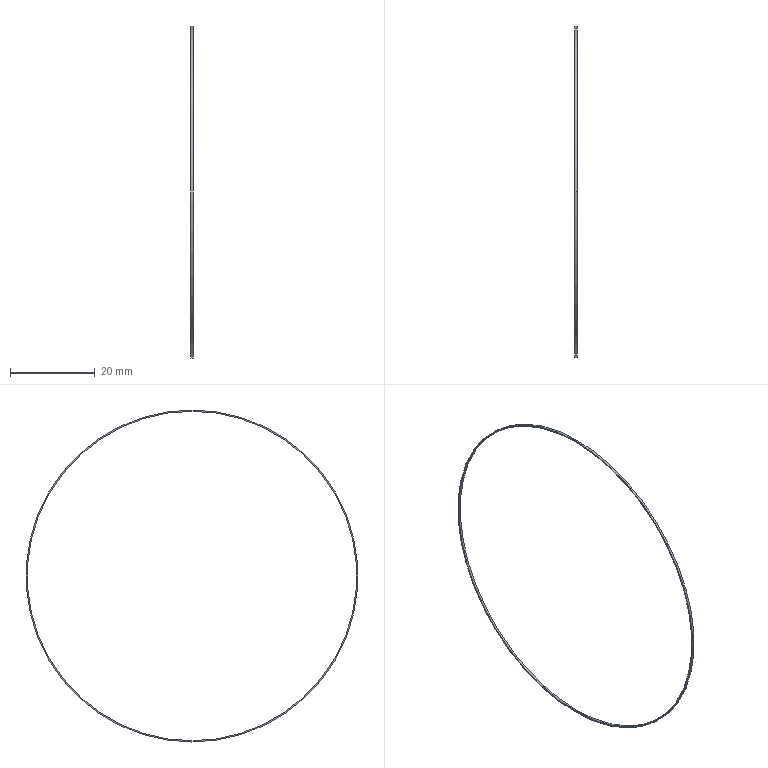Part | STEP file | USZCZELKA_SIMMERING1V11 | 1 solid | 6 faces | box 0.5 x 78.541 x 78.541 mm | volume 35.939 mm3 | cylinder 4 | plane 2 | commonest cylinder face diameters 77.956 x2 78.541 x2
STEP:
#1=CARTESIAN_POINT('',(0.,0.,0.));
#2=DIRECTION('',(0.,0.,1.));
#3=DIRECTION('',(1.,0.,0.));
#4=AXIS2_PLACEMENT_3D('',#1,#2,#3);
#5=CARTESIAN_POINT('',(0.25,0.,38.978));
#6=VERTEX_POINT('',#5);
#7=CARTESIAN_POINT('',(-0.25,0.,38.978));
#8=VERTEX_POINT('',#7);
#9=CARTESIAN_POINT('',(0.25,0.,38.978));
#10=DIRECTION('',(-1.,0.,0.));
#11=VECTOR('',#10,1.);
#12=LINE('',#9,#11);
#13=CARTESIAN_POINT('',(0.25,0.,0.));
#14=DIRECTION('',(-1.,0.,0.));
#15=DIRECTION('',(0.,0.,1.));
#16=AXIS2_PLACEMENT_3D('',#13,#14,#15);
#17=CYLINDRICAL_SURFACE('',#16,38.978);
#18=CARTESIAN_POINT('',(6.283,0.));
#19=DIRECTION('',(0.,1.));
#20=VECTOR('',#19,1.);
#21=LINE('',#18,#20);
#22=(GEOMETRIC_REPRESENTATION_CONTEXT(2)PARAMETRIC_REPRESENTATION_CONTEXT()REPRESENTATION_CONTEXT('',''));
#23=DEFINITIONAL_REPRESENTATION('',(#21),#22);
#24=PCURVE('',#17,#23);
#25=CARTESIAN_POINT('',(0.25,0.,0.));
#26=DIRECTION('',(-1.,0.,0.));
#27=DIRECTION('',(0.,0.,1.));
#28=AXIS2_PLACEMENT_3D('',#25,#26,#27);
#29=CYLINDRICAL_SURFACE('',#28,38.978);
#30=CARTESIAN_POINT('',(0.,0.));
#31=DIRECTION('',(0.,1.));
#32=VECTOR('',#31,1.);
#33=LINE('',#30,#32);
#34=(GEOMETRIC_REPRESENTATION_CONTEXT(2)PARAMETRIC_REPRESENTATION_CONTEXT()REPRESENTATION_CONTEXT('',''));
#35=DEFINITIONAL_REPRESENTATION('',(#33),#34);
#36=PCURVE('',#29,#35);
#37=SURFACE_CURVE('',#12,(#24,#36),.PCURVE_S1.);
#38=EDGE_CURVE('',#6,#8,#37,.T.);
#39=ORIENTED_EDGE('',*,*,#38,.T.);
#40=CARTESIAN_POINT('',(-0.25,0.,-38.978));
#41=VERTEX_POINT('',#40);
#42=CARTESIAN_POINT('',(-0.25,0.,0.));
#43=DIRECTION('',(1.,0.,0.));
#44=DIRECTION('',(0.,0.,-1.));
#45=AXIS2_PLACEMENT_3D('',#42,#43,#44);
#46=CIRCLE('',#45,38.978);
#47=CARTESIAN_POINT('',(9.425,0.5));
#48=DIRECTION('',(-1.,0.));
#49=VECTOR('',#48,1.);
#50=LINE('',#47,#49);
#51=(GEOMETRIC_REPRESENTATION_CONTEXT(2)PARAMETRIC_REPRESENTATION_CONTEXT()REPRESENTATION_CONTEXT('',''));
#52=DEFINITIONAL_REPRESENTATION('',(#50),#51);
#53=PCURVE('',#17,#52);
#54=CARTESIAN_POINT('',(-0.25,0.,0.));
#55=DIRECTION('',(1.,0.,0.));
#56=DIRECTION('',(0.,0.,-1.));
#57=AXIS2_PLACEMENT_3D('',#54,#55,#56);
#58=PLANE('',#57);
#59=CARTESIAN_POINT('',(0.,0.));
#60=DIRECTION('',(1.,0.));
#61=AXIS2_PLACEMENT_2D('',#59,#60);
#62=CIRCLE('',#61,38.978);
#63=(GEOMETRIC_REPRESENTATION_CONTEXT(2)PARAMETRIC_REPRESENTATION_CONTEXT()REPRESENTATION_CONTEXT('',''));
#64=DEFINITIONAL_REPRESENTATION('',(#62),#63);
#65=PCURVE('',#58,#64);
#66=SURFACE_CURVE('',#46,(#53,#65),.PCURVE_S1.);
#67=EDGE_CURVE('',#8,#41,#66,.T.);
#68=ORIENTED_EDGE('',*,*,#67,.T.);
#69=CARTESIAN_POINT('',(0.25,0.,-38.978));
#70=VERTEX_POINT('',#69);
#71=CARTESIAN_POINT('',(0.25,0.,-38.978));
#72=DIRECTION('',(-1.,0.,0.));
#73=VECTOR('',#72,1.);
#74=LINE('',#71,#73);
#75=CARTESIAN_POINT('',(3.142,0.));
#76=DIRECTION('',(0.,1.));
#77=VECTOR('',#76,1.);
#78=LINE('',#75,#77);
#79=(GEOMETRIC_REPRESENTATION_CONTEXT(2)PARAMETRIC_REPRESENTATION_CONTEXT()REPRESENTATION_CONTEXT('',''));
#80=DEFINITIONAL_REPRESENTATION('',(#78),#79);
#81=PCURVE('',#17,#80);
#82=CARTESIAN_POINT('',(3.142,0.));
#83=DIRECTION('',(0.,1.));
#84=VECTOR('',#83,1.);
#85=LINE('',#82,#84);
#86=(GEOMETRIC_REPRESENTATION_CONTEXT(2)PARAMETRIC_REPRESENTATION_CONTEXT()REPRESENTATION_CONTEXT('',''));
#87=DEFINITIONAL_REPRESENTATION('',(#85),#86);
#88=PCURVE('',#29,#87);
#89=SURFACE_CURVE('',#74,(#81,#88),.PCURVE_S1.);
#90=EDGE_CURVE('',#70,#41,#89,.T.);
#91=ORIENTED_EDGE('',*,*,#90,.F.);
#92=CARTESIAN_POINT('',(0.25,0.,0.));
#93=DIRECTION('',(1.,0.,0.));
#94=DIRECTION('',(0.,0.,-1.));
#95=AXIS2_PLACEMENT_3D('',#92,#93,#94);
#96=CIRCLE('',#95,38.978);
#97=CARTESIAN_POINT('',(9.425,0.));
#98=DIRECTION('',(-1.,0.));
#99=VECTOR('',#98,1.);
#100=LINE('',#97,#99);
#101=(GEOMETRIC_REPRESENTATION_CONTEXT(2)PARAMETRIC_REPRESENTATION_CONTEXT()REPRESENTATION_CONTEXT('',''));
#102=DEFINITIONAL_REPRESENTATION('',(#100),#101);
#103=PCURVE('',#17,#102);
#104=CARTESIAN_POINT('',(0.25,0.,0.));
#105=DIRECTION('',(1.,0.,0.));
#106=DIRECTION('',(0.,0.,-1.));
#107=AXIS2_PLACEMENT_3D('',#104,#105,#106);
#108=PLANE('',#107);
#109=CARTESIAN_POINT('',(0.,0.));
#110=DIRECTION('',(1.,0.));
#111=AXIS2_PLACEMENT_2D('',#109,#110);
#112=CIRCLE('',#111,38.978);
#113=(GEOMETRIC_REPRESENTATION_CONTEXT(2)PARAMETRIC_REPRESENTATION_CONTEXT()REPRESENTATION_CONTEXT('',''));
#114=DEFINITIONAL_REPRESENTATION('',(#112),#113);
#115=PCURVE('',#108,#114);
#116=SURFACE_CURVE('',#96,(#103,#115),.PCURVE_S1.);
#117=EDGE_CURVE('',#6,#70,#116,.T.);
#118=ORIENTED_EDGE('',*,*,#117,.F.);
#119=EDGE_LOOP('',(#39,#68,#91,#118));
#120=FACE_BOUND('',#119,.F.);
#121=ADVANCED_FACE('',(#120),#17,.F.);
#122=CARTESIAN_POINT('',(0.25,0.,-39.27));
#123=VERTEX_POINT('',#122);
#124=CARTESIAN_POINT('',(0.25,0.,39.27));
#125=VERTEX_POINT('',#124);
#126=CARTESIAN_POINT('',(0.25,0.,0.));
#127=DIRECTION('',(1.,0.,0.));
#128=DIRECTION('',(0.,0.,-1.));
#129=AXIS2_PLACEMENT_3D('',#126,#127,#128);
#130=CIRCLE('',#129,39.27);
#131=CARTESIAN_POINT('',(0.25,0.,0.));
#132=DIRECTION('',(-1.,0.,0.));
#133=DIRECTION('',(0.,0.,1.));
#134=AXIS2_PLACEMENT_3D('',#131,#132,#133);
#135=CYLINDRICAL_SURFACE('',#134,39.27);
#136=CARTESIAN_POINT('',(3.142,0.));
#137=DIRECTION('',(-1.,0.));
#138=VECTOR('',#137,1.);
#139=LINE('',#136,#138);
#140=(GEOMETRIC_REPRESENTATION_CONTEXT(2)PARAMETRIC_REPRESENTATION_CONTEXT()REPRESENTATION_CONTEXT('',''));
#141=DEFINITIONAL_REPRESENTATION('',(#139),#140);
#142=PCURVE('',#135,#141);
#143=CARTESIAN_POINT('',(0.,0.));
#144=DIRECTION('',(1.,0.));
#145=AXIS2_PLACEMENT_2D('',#143,#144);
#146=CIRCLE('',#145,39.27);
#147=(GEOMETRIC_REPRESENTATION_CONTEXT(2)PARAMETRIC_REPRESENTATION_CONTEXT()REPRESENTATION_CONTEXT('',''));
#148=DEFINITIONAL_REPRESENTATION('',(#146),#147);
#149=PCURVE('',#108,#148);
#150=SURFACE_CURVE('',#130,(#142,#149),.PCURVE_S1.);
#151=EDGE_CURVE('',#123,#125,#150,.T.);
#152=ORIENTED_EDGE('',*,*,#151,.F.);
#153=CARTESIAN_POINT('',(-0.25,0.,-39.27));
#154=VERTEX_POINT('',#153);
#155=CARTESIAN_POINT('',(0.25,0.,-39.27));
#156=DIRECTION('',(-1.,0.,0.));
#157=VECTOR('',#156,1.);
#158=LINE('',#155,#157);
#159=CARTESIAN_POINT('',(3.142,0.));
#160=DIRECTION('',(0.,1.));
#161=VECTOR('',#160,1.);
#162=LINE('',#159,#161);
#163=(GEOMETRIC_REPRESENTATION_CONTEXT(2)PARAMETRIC_REPRESENTATION_CONTEXT()REPRESENTATION_CONTEXT('',''));
#164=DEFINITIONAL_REPRESENTATION('',(#162),#163);
#165=PCURVE('',#135,#164);
#166=CARTESIAN_POINT('',(0.25,0.,0.));
#167=DIRECTION('',(-1.,0.,0.));
#168=DIRECTION('',(0.,0.,1.));
#169=AXIS2_PLACEMENT_3D('',#166,#167,#168);
#170=CYLINDRICAL_SURFACE('',#169,39.27);
#171=CARTESIAN_POINT('',(3.142,0.));
#172=DIRECTION('',(0.,1.));
#173=VECTOR('',#172,1.);
#174=LINE('',#171,#173);
#175=(GEOMETRIC_REPRESENTATION_CONTEXT(2)PARAMETRIC_REPRESENTATION_CONTEXT()REPRESENTATION_CONTEXT('',''));
#176=DEFINITIONAL_REPRESENTATION('',(#174),#175);
#177=PCURVE('',#170,#176);
#178=SURFACE_CURVE('',#158,(#165,#177),.PCURVE_S1.);
#179=EDGE_CURVE('',#123,#154,#178,.T.);
#180=ORIENTED_EDGE('',*,*,#179,.T.);
#181=CARTESIAN_POINT('',(-0.25,0.,39.27));
#182=VERTEX_POINT('',#181);
#183=CARTESIAN_POINT('',(-0.25,0.,0.));
#184=DIRECTION('',(1.,0.,0.));
#185=DIRECTION('',(0.,0.,-1.));
#186=AXIS2_PLACEMENT_3D('',#183,#184,#185);
#187=CIRCLE('',#186,39.27);
#188=CARTESIAN_POINT('',(3.142,0.5));
#189=DIRECTION('',(-1.,0.));
#190=VECTOR('',#189,1.);
#191=LINE('',#188,#190);
#192=(GEOMETRIC_REPRESENTATION_CONTEXT(2)PARAMETRIC_REPRESENTATION_CONTEXT()REPRESENTATION_CONTEXT('',''));
#193=DEFINITIONAL_REPRESENTATION('',(#191),#192);
#194=PCURVE('',#135,#193);
#195=CARTESIAN_POINT('',(0.,0.));
#196=DIRECTION('',(1.,0.));
#197=AXIS2_PLACEMENT_2D('',#195,#196);
#198=CIRCLE('',#197,39.27);
#199=(GEOMETRIC_REPRESENTATION_CONTEXT(2)PARAMETRIC_REPRESENTATION_CONTEXT()REPRESENTATION_CONTEXT('',''));
#200=DEFINITIONAL_REPRESENTATION('',(#198),#199);
#201=PCURVE('',#58,#200);
#202=SURFACE_CURVE('',#187,(#194,#201),.PCURVE_S1.);
#203=EDGE_CURVE('',#154,#182,#202,.T.);
#204=ORIENTED_EDGE('',*,*,#203,.T.);
#205=CARTESIAN_POINT('',(0.25,0.,39.27));
#206=DIRECTION('',(-1.,0.,0.));
#207=VECTOR('',#206,1.);
#208=LINE('',#205,#207);
#209=CARTESIAN_POINT('',(0.,0.));
#210=DIRECTION('',(0.,1.));
#211=VECTOR('',#210,1.);
#212=LINE('',#209,#211);
#213=(GEOMETRIC_REPRESENTATION_CONTEXT(2)PARAMETRIC_REPRESENTATION_CONTEXT()REPRESENTATION_CONTEXT('',''));
#214=DEFINITIONAL_REPRESENTATION('',(#212),#213);
#215=PCURVE('',#135,#214);
#216=CARTESIAN_POINT('',(6.283,0.));
#217=DIRECTION('',(0.,1.));
#218=VECTOR('',#217,1.);
#219=LINE('',#216,#218);
#220=(GEOMETRIC_REPRESENTATION_CONTEXT(2)PARAMETRIC_REPRESENTATION_CONTEXT()REPRESENTATION_CONTEXT('',''));
#221=DEFINITIONAL_REPRESENTATION('',(#219),#220);
#222=PCURVE('',#170,#221);
#223=SURFACE_CURVE('',#208,(#215,#222),.PCURVE_S1.);
#224=EDGE_CURVE('',#125,#182,#223,.T.);
#225=ORIENTED_EDGE('',*,*,#224,.F.);
#226=EDGE_LOOP('',(#152,#180,#204,#225));
#227=FACE_BOUND('',#226,.T.);
#228=ADVANCED_FACE('',(#227),#135,.T.);
#229=CARTESIAN_POINT('',(0.25,0.,0.));
#230=DIRECTION('',(1.,0.,0.));
#231=DIRECTION('',(0.,0.,-1.));
#232=AXIS2_PLACEMENT_3D('',#229,#230,#231);
#233=CIRCLE('',#232,39.27);
#234=CARTESIAN_POINT('',(0.,0.));
#235=DIRECTION('',(1.,0.));
#236=AXIS2_PLACEMENT_2D('',#234,#235);
#237=CIRCLE('',#236,39.27);
#238=(GEOMETRIC_REPRESENTATION_CONTEXT(2)PARAMETRIC_REPRESENTATION_CONTEXT()REPRESENTATION_CONTEXT('',''));
#239=DEFINITIONAL_REPRESENTATION('',(#237),#238);
#240=PCURVE('',#108,#239);
#241=CARTESIAN_POINT('',(9.425,0.));
#242=DIRECTION('',(-1.,0.));
#243=VECTOR('',#242,1.);
#244=LINE('',#241,#243);
#245=(GEOMETRIC_REPRESENTATION_CONTEXT(2)PARAMETRIC_REPRESENTATION_CONTEXT()REPRESENTATION_CONTEXT('',''));
#246=DEFINITIONAL_REPRESENTATION('',(#244),#245);
#247=PCURVE('',#170,#246);
#248=SURFACE_CURVE('',#233,(#240,#247),.PCURVE_S1.);
#249=EDGE_CURVE('',#125,#123,#248,.T.);
#250=ORIENTED_EDGE('',*,*,#249,.T.);
#251=ORIENTED_EDGE('',*,*,#151,.T.);
#252=EDGE_LOOP('',(#250,#251));
#253=FACE_BOUND('',#252,.T.);
#254=ORIENTED_EDGE('',*,*,#117,.F.);
#255=CARTESIAN_POINT('',(0.25,0.,0.));
#256=DIRECTION('',(1.,0.,0.));
#257=DIRECTION('',(0.,0.,-1.));
#258=AXIS2_PLACEMENT_3D('',#255,#256,#257);
#259=CIRCLE('',#258,38.978);
#260=CARTESIAN_POINT('',(0.,0.));
#261=DIRECTION('',(1.,0.));
#262=AXIS2_PLACEMENT_2D('',#260,#261);
#263=CIRCLE('',#262,38.978);
#264=(GEOMETRIC_REPRESENTATION_CONTEXT(2)PARAMETRIC_REPRESENTATION_CONTEXT()REPRESENTATION_CONTEXT('',''));
#265=DEFINITIONAL_REPRESENTATION('',(#263),#264);
#266=PCURVE('',#108,#265);
#267=CARTESIAN_POINT('',(3.142,0.));
#268=DIRECTION('',(-1.,0.));
#269=VECTOR('',#268,1.);
#270=LINE('',#267,#269);
#271=(GEOMETRIC_REPRESENTATION_CONTEXT(2)PARAMETRIC_REPRESENTATION_CONTEXT()REPRESENTATION_CONTEXT('',''));
#272=DEFINITIONAL_REPRESENTATION('',(#270),#271);
#273=PCURVE('',#29,#272);
#274=SURFACE_CURVE('',#259,(#266,#273),.PCURVE_S1.);
#275=EDGE_CURVE('',#70,#6,#274,.T.);
#276=ORIENTED_EDGE('',*,*,#275,.F.);
#277=EDGE_LOOP('',(#254,#276));
#278=FACE_BOUND('',#277,.T.);
#279=ADVANCED_FACE('',(#253,#278),#108,.T.);
#280=CARTESIAN_POINT('',(-0.25,0.,0.));
#281=DIRECTION('',(1.,0.,0.));
#282=DIRECTION('',(0.,0.,-1.));
#283=AXIS2_PLACEMENT_3D('',#280,#281,#282);
#284=CIRCLE('',#283,39.27);
#285=CARTESIAN_POINT('',(0.,0.));
#286=DIRECTION('',(1.,0.));
#287=AXIS2_PLACEMENT_2D('',#285,#286);
#288=CIRCLE('',#287,39.27);
#289=(GEOMETRIC_REPRESENTATION_CONTEXT(2)PARAMETRIC_REPRESENTATION_CONTEXT()REPRESENTATION_CONTEXT('',''));
#290=DEFINITIONAL_REPRESENTATION('',(#288),#289);
#291=PCURVE('',#58,#290);
#292=CARTESIAN_POINT('',(9.425,0.5));
#293=DIRECTION('',(-1.,0.));
#294=VECTOR('',#293,1.);
#295=LINE('',#292,#294);
#296=(GEOMETRIC_REPRESENTATION_CONTEXT(2)PARAMETRIC_REPRESENTATION_CONTEXT()REPRESENTATION_CONTEXT('',''));
#297=DEFINITIONAL_REPRESENTATION('',(#295),#296);
#298=PCURVE('',#170,#297);
#299=SURFACE_CURVE('',#284,(#291,#298),.PCURVE_S1.);
#300=EDGE_CURVE('',#182,#154,#299,.T.);
#301=ORIENTED_EDGE('',*,*,#300,.F.);
#302=ORIENTED_EDGE('',*,*,#203,.F.);
#303=EDGE_LOOP('',(#301,#302));
#304=FACE_BOUND('',#303,.T.);
#305=ORIENTED_EDGE('',*,*,#67,.T.);
#306=CARTESIAN_POINT('',(-0.25,0.,0.));
#307=DIRECTION('',(1.,0.,0.));
#308=DIRECTION('',(0.,0.,-1.));
#309=AXIS2_PLACEMENT_3D('',#306,#307,#308);
#310=CIRCLE('',#309,38.978);
#311=CARTESIAN_POINT('',(0.,0.));
#312=DIRECTION('',(1.,0.));
#313=AXIS2_PLACEMENT_2D('',#311,#312);
#314=CIRCLE('',#313,38.978);
#315=(GEOMETRIC_REPRESENTATION_CONTEXT(2)PARAMETRIC_REPRESENTATION_CONTEXT()REPRESENTATION_CONTEXT('',''));
#316=DEFINITIONAL_REPRESENTATION('',(#314),#315);
#317=PCURVE('',#58,#316);
#318=CARTESIAN_POINT('',(3.142,0.5));
#319=DIRECTION('',(-1.,0.));
#320=VECTOR('',#319,1.);
#321=LINE('',#318,#320);
#322=(GEOMETRIC_REPRESENTATION_CONTEXT(2)PARAMETRIC_REPRESENTATION_CONTEXT()REPRESENTATION_CONTEXT('',''));
#323=DEFINITIONAL_REPRESENTATION('',(#321),#322);
#324=PCURVE('',#29,#323);
#325=SURFACE_CURVE('',#310,(#317,#324),.PCURVE_S1.);
#326=EDGE_CURVE('',#41,#8,#325,.T.);
#327=ORIENTED_EDGE('',*,*,#326,.T.);
#328=EDGE_LOOP('',(#305,#327));
#329=FACE_BOUND('',#328,.T.);
#330=ADVANCED_FACE('',(#304,#329),#58,.F.);
#331=ORIENTED_EDGE('',*,*,#179,.F.);
#332=ORIENTED_EDGE('',*,*,#249,.F.);
#333=ORIENTED_EDGE('',*,*,#224,.T.);
#334=ORIENTED_EDGE('',*,*,#300,.T.);
#335=EDGE_LOOP('',(#331,#332,#333,#334));
#336=FACE_BOUND('',#335,.T.);
#337=ADVANCED_FACE('',(#336),#170,.T.);
#338=ORIENTED_EDGE('',*,*,#326,.T.);
#339=ORIENTED_EDGE('',*,*,#38,.F.);
#340=ORIENTED_EDGE('',*,*,#275,.F.);
#341=ORIENTED_EDGE('',*,*,#90,.T.);
#342=EDGE_LOOP('',(#338,#339,#340,#341));
#343=FACE_BOUND('',#342,.F.);
#344=ADVANCED_FACE('',(#343),#29,.F.);
#345=CLOSED_SHELL('',(#121,#228,#279,#330,#337,#344));
#346=MANIFOLD_SOLID_BREP('',#345);
#347=(LENGTH_UNIT()NAMED_UNIT(*)SI_UNIT(.MILLI.,.METRE.));
#348=UNCERTAINTY_MEASURE_WITH_UNIT(LENGTH_MEASURE(0.0000001),#347,'','');
#349=(NAMED_UNIT(*)PLANE_ANGLE_UNIT()SI_UNIT($,.RADIAN.));
#350=(NAMED_UNIT(*)SI_UNIT($,.STERADIAN.)SOLID_ANGLE_UNIT());
#351=(GEOMETRIC_REPRESENTATION_CONTEXT(3)GLOBAL_UNCERTAINTY_ASSIGNED_CONTEXT((#348))GLOBAL_UNIT_ASSIGNED_CONTEXT((#347,#349,#350))REPRESENTATION_CONTEXT('',''));
#352=ADVANCED_BREP_SHAPE_REPRESENTATION('',(#4,#346),#351);